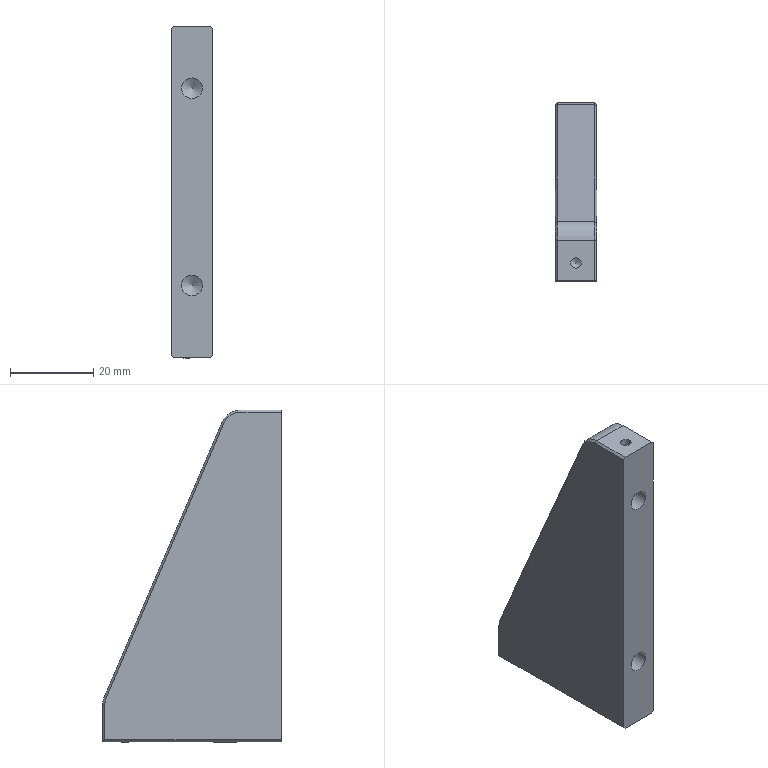Part | STEP file | ROTATION MC_NEW VER-0610_566 | 1 solid | 33 faces | box 10 x 43 x 80 mm | volume 22787 mm3 | plane 15 | cone 10 | cylinder 8 | commonest cylinder face diameters 5 x4 2.5 x2 10 x2
STEP:
#1=CARTESIAN_POINT('',(-187.469,717.468,-130.341));
#2=VERTEX_POINT('',#1);
#3=CARTESIAN_POINT('',(-187.469,717.468,-132.841));
#4=VERTEX_POINT('',#3);
#5=CARTESIAN_POINT('',(-187.469,717.468,-131.591));
#6=DIRECTION('',(0.,-1.,0.));
#7=DIRECTION('',(0.,0.,1.));
#8=AXIS2_PLACEMENT_3D('',#5,#6,#7);
#9=CIRCLE('',#8,1.25);
#10=EDGE_CURVE('',#2,#4,#9,.T.);
#11=ORIENTED_EDGE('',*,*,#10,.F.);
#12=CARTESIAN_POINT('',(-187.469,717.468,-131.591));
#13=DIRECTION('',(0.,-1.,0.));
#14=DIRECTION('',(0.,0.,1.));
#15=AXIS2_PLACEMENT_3D('',#12,#13,#14);
#16=CIRCLE('',#15,1.25);
#17=EDGE_CURVE('',#4,#2,#16,.T.);
#18=ORIENTED_EDGE('',*,*,#17,.F.);
#19=CARTESIAN_POINT('',(-187.469,712.468,-132.841));
#20=VERTEX_POINT('',#19);
#21=CARTESIAN_POINT('',(-187.469,717.468,-132.841));
#22=DIRECTION('',(0.,-1.,0.));
#23=VECTOR('',#22,1.25);
#24=LINE('',#21,#23);
#25=EDGE_CURVE('',#4,#20,#24,.T.);
#26=ORIENTED_EDGE('',*,*,#25,.T.);
#27=CARTESIAN_POINT('',(-187.469,712.468,-130.341));
#28=VERTEX_POINT('',#27);
#29=CARTESIAN_POINT('',(-187.469,712.468,-131.591));
#30=DIRECTION('',(0.,1.,0.));
#31=DIRECTION('',(0.,0.,1.));
#32=AXIS2_PLACEMENT_3D('',#29,#30,#31);
#33=CIRCLE('',#32,1.25);
#34=EDGE_CURVE('',#28,#20,#33,.T.);
#35=ORIENTED_EDGE('',*,*,#34,.F.);
#36=CARTESIAN_POINT('',(-187.469,712.468,-131.591));
#37=DIRECTION('',(0.,1.,0.));
#38=DIRECTION('',(0.,0.,1.));
#39=AXIS2_PLACEMENT_3D('',#36,#37,#38);
#40=CIRCLE('',#39,1.25);
#41=EDGE_CURVE('',#20,#28,#40,.T.);
#42=ORIENTED_EDGE('',*,*,#41,.F.);
#43=ORIENTED_EDGE('',*,*,#25,.F.);
#44=EDGE_LOOP('',(#11,#18,#26,#35,#42,#43));
#45=FACE_OUTER_BOUND('',#44,.T.);
#46=CARTESIAN_POINT('',(-187.469,717.468,-131.591));
#47=DIRECTION('',(0.,-1.,0.));
#48=DIRECTION('',(0.,0.,1.));
#49=AXIS2_PLACEMENT_3D('',#46,#47,#48);
#50=CYLINDRICAL_SURFACE('',#49,1.25);
#51=ADVANCED_FACE('',(#45),#50,.F.);
#52=CARTESIAN_POINT('',(-187.469,711.717,-131.591));
#53=VERTEX_POINT('',#52);
#54=CARTESIAN_POINT('',(-187.469,712.468,-130.341));
#55=DIRECTION('',(0.,0.515,0.8572));
#56=VECTOR('',#55,1.25);
#57=LINE('',#54,#56);
#58=EDGE_CURVE('',#53,#28,#57,.T.);
#59=ORIENTED_EDGE('',*,*,#58,.T.);
#60=ORIENTED_EDGE('',*,*,#34,.T.);
#61=ORIENTED_EDGE('',*,*,#41,.T.);
#62=ORIENTED_EDGE('',*,*,#58,.F.);
#63=EDGE_LOOP('',(#59,#60,#61,#62));
#64=FACE_OUTER_BOUND('',#63,.T.);
#65=CARTESIAN_POINT('',(-187.469,712.468,-131.591));
#66=DIRECTION('',(0.,1.,0.));
#67=DIRECTION('',(0.,0.,-1.));
#68=AXIS2_PLACEMENT_3D('',#65,#66,#67);
#69=CONICAL_SURFACE('',#68,1.25,1.03);
#70=ADVANCED_FACE('',(#64),#69,.F.);
#71=CARTESIAN_POINT('',(-187.469,685.468,-136.091));
#72=VERTEX_POINT('',#71);
#73=CARTESIAN_POINT('',(-187.469,680.468,-136.091));
#74=VERTEX_POINT('',#73);
#75=CARTESIAN_POINT('',(-187.469,682.968,-136.091));
#76=DIRECTION('',(0.,0.,1.));
#77=DIRECTION('',(0.,1.,0.));
#78=AXIS2_PLACEMENT_3D('',#75,#76,#77);
#79=CIRCLE('',#78,2.5);
#80=EDGE_CURVE('',#72,#74,#79,.T.);
#81=ORIENTED_EDGE('',*,*,#80,.F.);
#82=CARTESIAN_POINT('',(-187.469,682.968,-136.091));
#83=DIRECTION('',(0.,0.,1.));
#84=DIRECTION('',(0.,1.,0.));
#85=AXIS2_PLACEMENT_3D('',#82,#83,#84);
#86=CIRCLE('',#85,2.5);
#87=EDGE_CURVE('',#74,#72,#86,.T.);
#88=ORIENTED_EDGE('',*,*,#87,.F.);
#89=CARTESIAN_POINT('',(-187.469,680.468,-124.091));
#90=VERTEX_POINT('',#89);
#91=CARTESIAN_POINT('',(-187.469,680.468,-136.091));
#92=DIRECTION('',(0.,0.,1.));
#93=VECTOR('',#92,2.5);
#94=LINE('',#91,#93);
#95=EDGE_CURVE('',#74,#90,#94,.T.);
#96=ORIENTED_EDGE('',*,*,#95,.T.);
#97=CARTESIAN_POINT('',(-187.469,685.468,-124.091));
#98=VERTEX_POINT('',#97);
#99=CARTESIAN_POINT('',(-187.469,682.968,-124.091));
#100=DIRECTION('',(0.,0.,-1.));
#101=DIRECTION('',(0.,1.,0.));
#102=AXIS2_PLACEMENT_3D('',#99,#100,#101);
#103=CIRCLE('',#102,2.5);
#104=EDGE_CURVE('',#98,#90,#103,.T.);
#105=ORIENTED_EDGE('',*,*,#104,.F.);
#106=CARTESIAN_POINT('',(-187.469,682.968,-124.091));
#107=DIRECTION('',(0.,0.,-1.));
#108=DIRECTION('',(0.,1.,0.));
#109=AXIS2_PLACEMENT_3D('',#106,#107,#108);
#110=CIRCLE('',#109,2.5);
#111=EDGE_CURVE('',#90,#98,#110,.T.);
#112=ORIENTED_EDGE('',*,*,#111,.F.);
#113=ORIENTED_EDGE('',*,*,#95,.F.);
#114=EDGE_LOOP('',(#81,#88,#96,#105,#112,#113));
#115=FACE_OUTER_BOUND('',#114,.T.);
#116=CARTESIAN_POINT('',(-187.469,682.968,-136.091));
#117=DIRECTION('',(0.,0.,1.));
#118=DIRECTION('',(0.,1.,0.));
#119=AXIS2_PLACEMENT_3D('',#116,#117,#118);
#120=CYLINDRICAL_SURFACE('',#119,2.5);
#121=ADVANCED_FACE('',(#115),#120,.F.);
#122=CARTESIAN_POINT('',(-187.469,682.968,-122.589));
#123=VERTEX_POINT('',#122);
#124=CARTESIAN_POINT('',(-187.469,685.468,-124.091));
#125=DIRECTION('',(0.,0.8572,-0.515));
#126=VECTOR('',#125,2.5);
#127=LINE('',#124,#126);
#128=EDGE_CURVE('',#123,#98,#127,.T.);
#129=ORIENTED_EDGE('',*,*,#128,.T.);
#130=ORIENTED_EDGE('',*,*,#104,.T.);
#131=ORIENTED_EDGE('',*,*,#111,.T.);
#132=ORIENTED_EDGE('',*,*,#128,.F.);
#133=EDGE_LOOP('',(#129,#130,#131,#132));
#134=FACE_OUTER_BOUND('',#133,.T.);
#135=CARTESIAN_POINT('',(-187.469,682.968,-124.091));
#136=DIRECTION('',(0.,0.,-1.));
#137=DIRECTION('',(0.,-1.,0.));
#138=AXIS2_PLACEMENT_3D('',#135,#136,#137);
#139=CONICAL_SURFACE('',#138,2.5,1.03);
#140=ADVANCED_FACE('',(#134),#139,.F.);
#141=CARTESIAN_POINT('',(-187.469,711.468,-136.091));
#142=VERTEX_POINT('',#141);
#143=CARTESIAN_POINT('',(-187.469,706.468,-136.091));
#144=VERTEX_POINT('',#143);
#145=CARTESIAN_POINT('',(-187.469,708.968,-136.091));
#146=DIRECTION('',(0.,0.,1.));
#147=DIRECTION('',(0.,1.,0.));
#148=AXIS2_PLACEMENT_3D('',#145,#146,#147);
#149=CIRCLE('',#148,2.5);
#150=EDGE_CURVE('',#142,#144,#149,.T.);
#151=ORIENTED_EDGE('',*,*,#150,.F.);
#152=CARTESIAN_POINT('',(-187.469,708.968,-136.091));
#153=DIRECTION('',(0.,0.,1.));
#154=DIRECTION('',(0.,1.,0.));
#155=AXIS2_PLACEMENT_3D('',#152,#153,#154);
#156=CIRCLE('',#155,2.5);
#157=EDGE_CURVE('',#144,#142,#156,.T.);
#158=ORIENTED_EDGE('',*,*,#157,.F.);
#159=CARTESIAN_POINT('',(-187.469,706.468,-124.091));
#160=VERTEX_POINT('',#159);
#161=CARTESIAN_POINT('',(-187.469,706.468,-136.091));
#162=DIRECTION('',(0.,0.,1.));
#163=VECTOR('',#162,2.5);
#164=LINE('',#161,#163);
#165=EDGE_CURVE('',#144,#160,#164,.T.);
#166=ORIENTED_EDGE('',*,*,#165,.T.);
#167=CARTESIAN_POINT('',(-187.469,711.468,-124.091));
#168=VERTEX_POINT('',#167);
#169=CARTESIAN_POINT('',(-187.469,708.968,-124.091));
#170=DIRECTION('',(0.,0.,-1.));
#171=DIRECTION('',(0.,1.,0.));
#172=AXIS2_PLACEMENT_3D('',#169,#170,#171);
#173=CIRCLE('',#172,2.5);
#174=EDGE_CURVE('',#168,#160,#173,.T.);
#175=ORIENTED_EDGE('',*,*,#174,.F.);
#176=CARTESIAN_POINT('',(-187.469,708.968,-124.091));
#177=DIRECTION('',(0.,0.,-1.));
#178=DIRECTION('',(0.,1.,0.));
#179=AXIS2_PLACEMENT_3D('',#176,#177,#178);
#180=CIRCLE('',#179,2.5);
#181=EDGE_CURVE('',#160,#168,#180,.T.);
#182=ORIENTED_EDGE('',*,*,#181,.F.);
#183=ORIENTED_EDGE('',*,*,#165,.F.);
#184=EDGE_LOOP('',(#151,#158,#166,#175,#182,#183));
#185=FACE_OUTER_BOUND('',#184,.T.);
#186=CARTESIAN_POINT('',(-187.469,708.968,-136.091));
#187=DIRECTION('',(0.,0.,1.));
#188=DIRECTION('',(0.,1.,0.));
#189=AXIS2_PLACEMENT_3D('',#186,#187,#188);
#190=CYLINDRICAL_SURFACE('',#189,2.5);
#191=ADVANCED_FACE('',(#185),#190,.F.);
#192=CARTESIAN_POINT('',(-187.469,708.968,-122.589));
#193=VERTEX_POINT('',#192);
#194=CARTESIAN_POINT('',(-187.469,711.468,-124.091));
#195=DIRECTION('',(0.,0.8572,-0.515));
#196=VECTOR('',#195,2.5);
#197=LINE('',#194,#196);
#198=EDGE_CURVE('',#193,#168,#197,.T.);
#199=ORIENTED_EDGE('',*,*,#198,.T.);
#200=ORIENTED_EDGE('',*,*,#174,.T.);
#201=ORIENTED_EDGE('',*,*,#181,.T.);
#202=ORIENTED_EDGE('',*,*,#198,.F.);
#203=EDGE_LOOP('',(#199,#200,#201,#202));
#204=FACE_OUTER_BOUND('',#203,.T.);
#205=CARTESIAN_POINT('',(-187.469,708.968,-124.091));
#206=DIRECTION('',(0.,0.,-1.));
#207=DIRECTION('',(0.,-1.,0.));
#208=AXIS2_PLACEMENT_3D('',#205,#206,#207);
#209=CONICAL_SURFACE('',#208,2.5,1.03);
#210=ADVANCED_FACE('',(#204),#209,.F.);
#211=CARTESIAN_POINT('',(-187.469,674.468,-121.091));
#212=VERTEX_POINT('',#211);
#213=CARTESIAN_POINT('',(-187.469,674.468,-116.091));
#214=VERTEX_POINT('',#213);
#215=CARTESIAN_POINT('',(-187.469,674.468,-118.591));
#216=DIRECTION('',(0.,1.,0.));
#217=DIRECTION('',(0.,0.,-1.));
#218=AXIS2_PLACEMENT_3D('',#215,#216,#217);
#219=CIRCLE('',#218,2.5);
#220=EDGE_CURVE('',#212,#214,#219,.T.);
#221=ORIENTED_EDGE('',*,*,#220,.F.);
#222=CARTESIAN_POINT('',(-187.469,674.468,-118.591));
#223=DIRECTION('',(0.,1.,0.));
#224=DIRECTION('',(0.,0.,-1.));
#225=AXIS2_PLACEMENT_3D('',#222,#223,#224);
#226=CIRCLE('',#225,2.5);
#227=EDGE_CURVE('',#214,#212,#226,.T.);
#228=ORIENTED_EDGE('',*,*,#227,.F.);
#229=CARTESIAN_POINT('',(-187.469,686.468,-116.091));
#230=VERTEX_POINT('',#229);
#231=CARTESIAN_POINT('',(-187.469,674.468,-116.091));
#232=DIRECTION('',(0.,1.,0.));
#233=VECTOR('',#232,2.5);
#234=LINE('',#231,#233);
#235=EDGE_CURVE('',#214,#230,#234,.T.);
#236=ORIENTED_EDGE('',*,*,#235,.T.);
#237=CARTESIAN_POINT('',(-187.469,686.468,-121.091));
#238=VERTEX_POINT('',#237);
#239=CARTESIAN_POINT('',(-187.469,686.468,-118.591));
#240=DIRECTION('',(0.,-1.,0.));
#241=DIRECTION('',(0.,0.,-1.));
#242=AXIS2_PLACEMENT_3D('',#239,#240,#241);
#243=CIRCLE('',#242,2.5);
#244=EDGE_CURVE('',#238,#230,#243,.T.);
#245=ORIENTED_EDGE('',*,*,#244,.F.);
#246=CARTESIAN_POINT('',(-187.469,686.468,-118.591));
#247=DIRECTION('',(0.,-1.,0.));
#248=DIRECTION('',(0.,0.,-1.));
#249=AXIS2_PLACEMENT_3D('',#246,#247,#248);
#250=CIRCLE('',#249,2.5);
#251=EDGE_CURVE('',#230,#238,#250,.T.);
#252=ORIENTED_EDGE('',*,*,#251,.F.);
#253=ORIENTED_EDGE('',*,*,#235,.F.);
#254=EDGE_LOOP('',(#221,#228,#236,#245,#252,#253));
#255=FACE_OUTER_BOUND('',#254,.T.);
#256=CARTESIAN_POINT('',(-187.469,674.468,-118.591));
#257=DIRECTION('',(0.,1.,0.));
#258=DIRECTION('',(0.,0.,-1.));
#259=AXIS2_PLACEMENT_3D('',#256,#257,#258);
#260=CYLINDRICAL_SURFACE('',#259,2.5);
#261=ADVANCED_FACE('',(#255),#260,.F.);
#262=CARTESIAN_POINT('',(-187.469,687.971,-118.591));
#263=VERTEX_POINT('',#262);
#264=CARTESIAN_POINT('',(-187.469,686.468,-121.091));
#265=DIRECTION('',(0.,-0.515,-0.8572));
#266=VECTOR('',#265,2.5);
#267=LINE('',#264,#266);
#268=EDGE_CURVE('',#263,#238,#267,.T.);
#269=ORIENTED_EDGE('',*,*,#268,.T.);
#270=ORIENTED_EDGE('',*,*,#244,.T.);
#271=ORIENTED_EDGE('',*,*,#251,.T.);
#272=ORIENTED_EDGE('',*,*,#268,.F.);
#273=EDGE_LOOP('',(#269,#270,#271,#272));
#274=FACE_OUTER_BOUND('',#273,.T.);
#275=CARTESIAN_POINT('',(-187.469,686.468,-118.591));
#276=DIRECTION('',(0.,-1.,0.));
#277=DIRECTION('',(0.,0.,1.));
#278=AXIS2_PLACEMENT_3D('',#275,#276,#277);
#279=CONICAL_SURFACE('',#278,2.5,1.03);
#280=ADVANCED_FACE('',(#274),#279,.F.);
#281=CARTESIAN_POINT('',(-187.469,674.468,-73.591));
#282=VERTEX_POINT('',#281);
#283=CARTESIAN_POINT('',(-187.469,674.468,-68.591));
#284=VERTEX_POINT('',#283);
#285=CARTESIAN_POINT('',(-187.469,674.468,-71.091));
#286=DIRECTION('',(0.,1.,0.));
#287=DIRECTION('',(0.,0.,-1.));
#288=AXIS2_PLACEMENT_3D('',#285,#286,#287);
#289=CIRCLE('',#288,2.5);
#290=EDGE_CURVE('',#282,#284,#289,.T.);
#291=ORIENTED_EDGE('',*,*,#290,.F.);
#292=CARTESIAN_POINT('',(-187.469,674.468,-71.091));
#293=DIRECTION('',(0.,1.,0.));
#294=DIRECTION('',(0.,0.,-1.));
#295=AXIS2_PLACEMENT_3D('',#292,#293,#294);
#296=CIRCLE('',#295,2.5);
#297=EDGE_CURVE('',#284,#282,#296,.T.);
#298=ORIENTED_EDGE('',*,*,#297,.F.);
#299=CARTESIAN_POINT('',(-187.469,686.468,-68.591));
#300=VERTEX_POINT('',#299);
#301=CARTESIAN_POINT('',(-187.469,674.468,-68.591));
#302=DIRECTION('',(0.,1.,0.));
#303=VECTOR('',#302,2.5);
#304=LINE('',#301,#303);
#305=EDGE_CURVE('',#284,#300,#304,.T.);
#306=ORIENTED_EDGE('',*,*,#305,.T.);
#307=CARTESIAN_POINT('',(-187.469,686.468,-73.591));
#308=VERTEX_POINT('',#307);
#309=CARTESIAN_POINT('',(-187.469,686.468,-71.091));
#310=DIRECTION('',(0.,-1.,0.));
#311=DIRECTION('',(0.,0.,-1.));
#312=AXIS2_PLACEMENT_3D('',#309,#310,#311);
#313=CIRCLE('',#312,2.5);
#314=EDGE_CURVE('',#308,#300,#313,.T.);
#315=ORIENTED_EDGE('',*,*,#314,.F.);
#316=CARTESIAN_POINT('',(-187.469,686.468,-71.091));
#317=DIRECTION('',(0.,-1.,0.));
#318=DIRECTION('',(0.,0.,-1.));
#319=AXIS2_PLACEMENT_3D('',#316,#317,#318);
#320=CIRCLE('',#319,2.5);
#321=EDGE_CURVE('',#300,#308,#320,.T.);
#322=ORIENTED_EDGE('',*,*,#321,.F.);
#323=ORIENTED_EDGE('',*,*,#305,.F.);
#324=EDGE_LOOP('',(#291,#298,#306,#315,#322,#323));
#325=FACE_OUTER_BOUND('',#324,.T.);
#326=CARTESIAN_POINT('',(-187.469,674.468,-71.091));
#327=DIRECTION('',(0.,1.,0.));
#328=DIRECTION('',(0.,0.,-1.));
#329=AXIS2_PLACEMENT_3D('',#326,#327,#328);
#330=CYLINDRICAL_SURFACE('',#329,2.5);
#331=ADVANCED_FACE('',(#325),#330,.F.);
#332=CARTESIAN_POINT('',(-187.469,687.971,-71.091));
#333=VERTEX_POINT('',#332);
#334=CARTESIAN_POINT('',(-187.469,686.468,-73.591));
#335=DIRECTION('',(0.,-0.515,-0.8572));
#336=VECTOR('',#335,2.5);
#337=LINE('',#334,#336);
#338=EDGE_CURVE('',#333,#308,#337,.T.);
#339=ORIENTED_EDGE('',*,*,#338,.T.);
#340=ORIENTED_EDGE('',*,*,#314,.T.);
#341=ORIENTED_EDGE('',*,*,#321,.T.);
#342=ORIENTED_EDGE('',*,*,#338,.F.);
#343=EDGE_LOOP('',(#339,#340,#341,#342));
#344=FACE_OUTER_BOUND('',#343,.T.);
#345=CARTESIAN_POINT('',(-187.469,686.468,-71.091));
#346=DIRECTION('',(0.,-1.,0.));
#347=DIRECTION('',(0.,0.,1.));
#348=AXIS2_PLACEMENT_3D('',#345,#346,#347);
#349=CONICAL_SURFACE('',#348,2.5,1.03);
#350=ADVANCED_FACE('',(#344),#349,.F.);
#351=CARTESIAN_POINT('',(-186.219,678.718,-56.091));
#352=VERTEX_POINT('',#351);
#353=CARTESIAN_POINT('',(-188.719,678.718,-56.091));
#354=VERTEX_POINT('',#353);
#355=CARTESIAN_POINT('',(-187.469,678.718,-56.091));
#356=DIRECTION('',(0.,0.,-1.));
#357=DIRECTION('',(1.,0.,0.));
#358=AXIS2_PLACEMENT_3D('',#355,#356,#357);
#359=CIRCLE('',#358,1.25);
#360=EDGE_CURVE('',#352,#354,#359,.T.);
#361=ORIENTED_EDGE('',*,*,#360,.F.);
#362=CARTESIAN_POINT('',(-187.469,678.718,-56.091));
#363=DIRECTION('',(0.,0.,-1.));
#364=DIRECTION('',(1.,0.,0.));
#365=AXIS2_PLACEMENT_3D('',#362,#363,#364);
#366=CIRCLE('',#365,1.25);
#367=EDGE_CURVE('',#354,#352,#366,.T.);
#368=ORIENTED_EDGE('',*,*,#367,.F.);
#369=CARTESIAN_POINT('',(-188.719,678.718,-66.091));
#370=VERTEX_POINT('',#369);
#371=CARTESIAN_POINT('',(-188.719,678.718,-56.091));
#372=DIRECTION('',(0.,0.,-1.));
#373=VECTOR('',#372,1.25);
#374=LINE('',#371,#373);
#375=EDGE_CURVE('',#354,#370,#374,.T.);
#376=ORIENTED_EDGE('',*,*,#375,.T.);
#377=CARTESIAN_POINT('',(-186.219,678.718,-66.091));
#378=VERTEX_POINT('',#377);
#379=CARTESIAN_POINT('',(-187.469,678.718,-66.091));
#380=DIRECTION('',(0.,0.,1.));
#381=DIRECTION('',(1.,0.,0.));
#382=AXIS2_PLACEMENT_3D('',#379,#380,#381);
#383=CIRCLE('',#382,1.25);
#384=EDGE_CURVE('',#378,#370,#383,.T.);
#385=ORIENTED_EDGE('',*,*,#384,.F.);
#386=CARTESIAN_POINT('',(-187.469,678.718,-66.091));
#387=DIRECTION('',(0.,0.,1.));
#388=DIRECTION('',(1.,0.,0.));
#389=AXIS2_PLACEMENT_3D('',#386,#387,#388);
#390=CIRCLE('',#389,1.25);
#391=EDGE_CURVE('',#370,#378,#390,.T.);
#392=ORIENTED_EDGE('',*,*,#391,.F.);
#393=ORIENTED_EDGE('',*,*,#375,.F.);
#394=EDGE_LOOP('',(#361,#368,#376,#385,#392,#393));
#395=FACE_OUTER_BOUND('',#394,.T.);
#396=CARTESIAN_POINT('',(-187.469,678.718,-56.091));
#397=DIRECTION('',(0.,0.,-1.));
#398=DIRECTION('',(1.,0.,0.));
#399=AXIS2_PLACEMENT_3D('',#396,#397,#398);
#400=CYLINDRICAL_SURFACE('',#399,1.25);
#401=ADVANCED_FACE('',(#395),#400,.F.);
#402=CARTESIAN_POINT('',(-187.469,678.718,-66.842));
#403=VERTEX_POINT('',#402);
#404=CARTESIAN_POINT('',(-186.219,678.718,-66.091));
#405=DIRECTION('',(0.8572,0.,0.515));
#406=VECTOR('',#405,1.25);
#407=LINE('',#404,#406);
#408=EDGE_CURVE('',#403,#378,#407,.T.);
#409=ORIENTED_EDGE('',*,*,#408,.T.);
#410=ORIENTED_EDGE('',*,*,#384,.T.);
#411=ORIENTED_EDGE('',*,*,#391,.T.);
#412=ORIENTED_EDGE('',*,*,#408,.F.);
#413=EDGE_LOOP('',(#409,#410,#411,#412));
#414=FACE_OUTER_BOUND('',#413,.T.);
#415=CARTESIAN_POINT('',(-187.469,678.718,-66.091));
#416=DIRECTION('',(0.,0.,1.));
#417=DIRECTION('',(-1.,0.,0.));
#418=AXIS2_PLACEMENT_3D('',#415,#416,#417);
#419=CONICAL_SURFACE('',#418,1.25,1.03);
#420=ADVANCED_FACE('',(#414),#419,.F.);
#421=CARTESIAN_POINT('',(-182.969,674.468,-56.091));
#422=VERTEX_POINT('',#421);
#423=CARTESIAN_POINT('',(-182.969,684.171,-56.091));
#424=VERTEX_POINT('',#423);
#425=CARTESIAN_POINT('',(-182.969,674.468,-56.091));
#426=DIRECTION('',(0.,1.,0.));
#427=VECTOR('',#426,9.703);
#428=LINE('',#425,#427);
#429=EDGE_CURVE('',#422,#424,#428,.T.);
#430=ORIENTED_EDGE('',*,*,#429,.T.);
#431=CARTESIAN_POINT('',(-191.969,684.171,-56.091));
#432=VERTEX_POINT('',#431);
#433=CARTESIAN_POINT('',(-191.969,684.171,-56.091));
#434=DIRECTION('',(1.,0.,0.));
#435=VECTOR('',#434,9.);
#436=LINE('',#433,#435);
#437=EDGE_CURVE('',#432,#424,#436,.T.);
#438=ORIENTED_EDGE('',*,*,#437,.F.);
#439=CARTESIAN_POINT('',(-191.969,674.468,-56.091));
#440=VERTEX_POINT('',#439);
#441=CARTESIAN_POINT('',(-191.969,684.171,-56.091));
#442=DIRECTION('',(0.,-1.,0.));
#443=VECTOR('',#442,9.703);
#444=LINE('',#441,#443);
#445=EDGE_CURVE('',#432,#440,#444,.T.);
#446=ORIENTED_EDGE('',*,*,#445,.T.);
#447=CARTESIAN_POINT('',(-191.969,674.468,-56.091));
#448=DIRECTION('',(1.,0.,0.));
#449=VECTOR('',#448,9.);
#450=LINE('',#447,#449);
#451=EDGE_CURVE('',#440,#422,#450,.T.);
#452=ORIENTED_EDGE('',*,*,#451,.T.);
#453=EDGE_LOOP('',(#430,#438,#446,#452));
#454=FACE_OUTER_BOUND('',#453,.T.);
#455=ORIENTED_EDGE('',*,*,#360,.T.);
#456=ORIENTED_EDGE('',*,*,#367,.T.);
#457=EDGE_LOOP('',(#455,#456));
#458=FACE_BOUND('',#457,.T.);
#459=CARTESIAN_POINT('',(-179.469,848.159,-56.091));
#460=DIRECTION('',(0.,0.,1.));
#461=DIRECTION('',(1.,0.,0.));
#462=AXIS2_PLACEMENT_3D('',#459,#460,#461);
#463=PLANE('',#462);
#464=ADVANCED_FACE('',(#454,#458),#463,.T.);
#465=CARTESIAN_POINT('',(-182.469,674.468,-56.591));
#466=VERTEX_POINT('',#465);
#467=CARTESIAN_POINT('',(-182.469,674.468,-56.591));
#468=DIRECTION('',(-0.7071,0.,0.7071));
#469=VECTOR('',#468,0.7071);
#470=LINE('',#467,#469);
#471=EDGE_CURVE('',#466,#422,#470,.T.);
#472=ORIENTED_EDGE('',*,*,#471,.F.);
#473=CARTESIAN_POINT('',(-182.469,684.171,-56.591));
#474=VERTEX_POINT('',#473);
#475=CARTESIAN_POINT('',(-182.469,684.171,-56.591));
#476=DIRECTION('',(0.,-1.,0.));
#477=VECTOR('',#476,9.703);
#478=LINE('',#475,#477);
#479=EDGE_CURVE('',#474,#466,#478,.T.);
#480=ORIENTED_EDGE('',*,*,#479,.F.);
#481=CARTESIAN_POINT('',(-182.969,684.171,-56.091));
#482=DIRECTION('',(0.7071,0.,-0.7071));
#483=VECTOR('',#482,0.7071);
#484=LINE('',#481,#483);
#485=EDGE_CURVE('',#424,#474,#484,.T.);
#486=ORIENTED_EDGE('',*,*,#485,.F.);
#487=ORIENTED_EDGE('',*,*,#429,.F.);
#488=EDGE_LOOP('',(#472,#480,#486,#487));
#489=FACE_OUTER_BOUND('',#488,.T.);
#490=CARTESIAN_POINT('',(-182.719,755.409,-56.341));
#491=DIRECTION('',(0.7071,0.,0.7071));
#492=DIRECTION('',(0.7071,0.,-0.7071));
#493=AXIS2_PLACEMENT_3D('',#490,#491,#492);
#494=PLANE('',#493);
#495=ADVANCED_FACE('',(#489),#494,.T.);
#496=ORIENTED_EDGE('',*,*,#471,.T.);
#497=ORIENTED_EDGE('',*,*,#451,.F.);
#498=CARTESIAN_POINT('',(-192.469,674.468,-56.591));
#499=VERTEX_POINT('',#498);
#500=CARTESIAN_POINT('',(-191.969,674.468,-56.091));
#501=DIRECTION('',(-0.7071,0.,-0.7071));
#502=VECTOR('',#501,0.7071);
#503=LINE('',#500,#502);
#504=EDGE_CURVE('',#440,#499,#503,.T.);
#505=ORIENTED_EDGE('',*,*,#504,.T.);
#506=CARTESIAN_POINT('',(-192.469,674.468,-135.591));
#507=VERTEX_POINT('',#506);
#508=CARTESIAN_POINT('',(-192.469,674.468,-135.591));
#509=DIRECTION('',(0.,0.,1.));
#510=VECTOR('',#509,79.);
#511=LINE('',#508,#510);
#512=EDGE_CURVE('',#507,#499,#511,.T.);
#513=ORIENTED_EDGE('',*,*,#512,.F.);
#514=CARTESIAN_POINT('',(-191.969,674.468,-136.091));
#515=VERTEX_POINT('',#514);
#516=CARTESIAN_POINT('',(-192.469,674.468,-135.591));
#517=DIRECTION('',(0.7071,0.,-0.7071));
#518=VECTOR('',#517,0.7071);
#519=LINE('',#516,#518);
#520=EDGE_CURVE('',#507,#515,#519,.T.);
#521=ORIENTED_EDGE('',*,*,#520,.T.);
#522=CARTESIAN_POINT('',(-182.969,674.468,-136.091));
#523=VERTEX_POINT('',#522);
#524=CARTESIAN_POINT('',(-182.969,674.468,-136.091));
#525=DIRECTION('',(-1.,0.,0.));
#526=VECTOR('',#525,9.);
#527=LINE('',#524,#526);
#528=EDGE_CURVE('',#523,#515,#527,.T.);
#529=ORIENTED_EDGE('',*,*,#528,.F.);
#530=CARTESIAN_POINT('',(-182.469,674.468,-135.591));
#531=VERTEX_POINT('',#530);
#532=CARTESIAN_POINT('',(-182.969,674.468,-136.091));
#533=DIRECTION('',(0.7071,0.,0.7071));
#534=VECTOR('',#533,0.7071);
#535=LINE('',#532,#534);
#536=EDGE_CURVE('',#523,#531,#535,.T.);
#537=ORIENTED_EDGE('',*,*,#536,.T.);
#538=CARTESIAN_POINT('',(-182.469,674.468,-56.591));
#539=DIRECTION('',(0.,0.,-1.));
#540=VECTOR('',#539,79.);
#541=LINE('',#538,#540);
#542=EDGE_CURVE('',#466,#531,#541,.T.);
#543=ORIENTED_EDGE('',*,*,#542,.F.);
#544=EDGE_LOOP('',(#496,#497,#505,#513,#521,#529,#537,#543));
#545=FACE_OUTER_BOUND('',#544,.T.);
#546=ORIENTED_EDGE('',*,*,#290,.T.);
#547=ORIENTED_EDGE('',*,*,#297,.T.);
#548=EDGE_LOOP('',(#546,#547));
#549=FACE_BOUND('',#548,.T.);
#550=ORIENTED_EDGE('',*,*,#220,.T.);
#551=ORIENTED_EDGE('',*,*,#227,.T.);
#552=EDGE_LOOP('',(#550,#551));
#553=FACE_BOUND('',#552,.T.);
#554=CARTESIAN_POINT('',(-179.469,674.468,-102.091));
#555=DIRECTION('',(0.,-1.,0.));
#556=DIRECTION('',(0.,0.,-1.));
#557=AXIS2_PLACEMENT_3D('',#554,#555,#556);
#558=PLANE('',#557);
#559=ADVANCED_FACE('',(#545,#549,#553),#558,.T.);
#560=ORIENTED_EDGE('',*,*,#479,.T.);
#561=ORIENTED_EDGE('',*,*,#542,.T.);
#562=CARTESIAN_POINT('',(-182.469,716.968,-135.591));
#563=VERTEX_POINT('',#562);
#564=CARTESIAN_POINT('',(-182.469,674.468,-135.591));
#565=DIRECTION('',(0.,1.,0.));
#566=VECTOR('',#565,42.5);
#567=LINE('',#564,#566);
#568=EDGE_CURVE('',#531,#563,#567,.T.);
#569=ORIENTED_EDGE('',*,*,#568,.T.);
#570=CARTESIAN_POINT('',(-182.469,716.968,-127.118));
#571=VERTEX_POINT('',#570);
#572=CARTESIAN_POINT('',(-182.469,716.968,-135.591));
#573=DIRECTION('',(0.,0.,1.));
#574=VECTOR('',#573,8.474);
#575=LINE('',#572,#574);
#576=EDGE_CURVE('',#563,#571,#575,.T.);
#577=ORIENTED_EDGE('',*,*,#576,.T.);
#578=CARTESIAN_POINT('',(-182.469,716.605,-125.345));
#579=VERTEX_POINT('',#578);
#580=CARTESIAN_POINT('',(-182.469,712.468,-127.118));
#581=DIRECTION('',(1.,0.,0.));
#582=DIRECTION('',(0.,1.,0.));
#583=AXIS2_PLACEMENT_3D('',#580,#581,#582);
#584=CIRCLE('',#583,4.5);
#585=EDGE_CURVE('',#571,#579,#584,.T.);
#586=ORIENTED_EDGE('',*,*,#585,.T.);
#587=CARTESIAN_POINT('',(-182.469,688.308,-59.319));
#588=VERTEX_POINT('',#587);
#589=CARTESIAN_POINT('',(-182.469,716.605,-125.345));
#590=DIRECTION('',(0.,-0.3939,0.9191));
#591=VECTOR('',#590,71.834);
#592=LINE('',#589,#591);
#593=EDGE_CURVE('',#579,#588,#592,.T.);
#594=ORIENTED_EDGE('',*,*,#593,.T.);
#595=CARTESIAN_POINT('',(-182.469,684.171,-61.091));
#596=DIRECTION('',(1.,0.,0.));
#597=DIRECTION('',(0.,0.9191,0.3939));
#598=AXIS2_PLACEMENT_3D('',#595,#596,#597);
#599=CIRCLE('',#598,4.5);
#600=EDGE_CURVE('',#588,#474,#599,.T.);
#601=ORIENTED_EDGE('',*,*,#600,.T.);
#602=EDGE_LOOP('',(#560,#561,#569,#577,#586,#594,#601));
#603=FACE_OUTER_BOUND('',#602,.T.);
#604=CARTESIAN_POINT('',(-182.469,662.659,-65.591));
#605=DIRECTION('',(-1.,0.,0.));
#606=DIRECTION('',(0.,0.,1.));
#607=AXIS2_PLACEMENT_3D('',#604,#605,#606);
#608=PLANE('',#607);
#609=ADVANCED_FACE('',(#603),#608,.F.);
#610=ORIENTED_EDGE('',*,*,#600,.F.);
#611=CARTESIAN_POINT('',(-182.969,688.767,-59.122));
#612=VERTEX_POINT('',#611);
#613=CARTESIAN_POINT('',(-182.969,688.767,-59.122));
#614=DIRECTION('',(0.7071,-0.6499,-0.2785));
#615=VECTOR('',#614,0.7071);
#616=LINE('',#613,#615);
#617=EDGE_CURVE('',#612,#588,#616,.T.);
#618=ORIENTED_EDGE('',*,*,#617,.F.);
#619=CARTESIAN_POINT('',(-182.969,684.171,-61.091));
#620=DIRECTION('',(1.,0.,0.));
#621=DIRECTION('',(0.,0.5505,0.8348));
#622=AXIS2_PLACEMENT_3D('',#619,#620,#621);
#623=CIRCLE('',#622,5.);
#624=EDGE_CURVE('',#612,#424,#623,.T.);
#625=ORIENTED_EDGE('',*,*,#624,.T.);
#626=ORIENTED_EDGE('',*,*,#485,.T.);
#627=EDGE_LOOP('',(#610,#618,#625,#626));
#628=FACE_OUTER_BOUND('',#627,.T.);
#629=CARTESIAN_POINT('',(-178.969,684.171,-61.091));
#630=DIRECTION('',(-1.,0.,0.));
#631=DIRECTION('',(0.,0.5505,0.8348));
#632=AXIS2_PLACEMENT_3D('',#629,#630,#631);
#633=CONICAL_SURFACE('',#632,1.,0.7854);
#634=ADVANCED_FACE('',(#628),#633,.T.);
#635=CARTESIAN_POINT('',(-191.969,688.767,-59.122));
#636=VERTEX_POINT('',#635);
#637=CARTESIAN_POINT('',(-191.969,684.171,-61.091));
#638=DIRECTION('',(-1.,0.,0.));
#639=DIRECTION('',(0.,0.5505,0.8348));
#640=AXIS2_PLACEMENT_3D('',#637,#638,#639);
#641=CIRCLE('',#640,5.);
#642=EDGE_CURVE('',#432,#636,#641,.T.);
#643=ORIENTED_EDGE('',*,*,#642,.F.);
#644=ORIENTED_EDGE('',*,*,#437,.T.);
#645=ORIENTED_EDGE('',*,*,#624,.F.);
#646=CARTESIAN_POINT('',(-182.969,688.767,-59.122));
#647=DIRECTION('',(-1.,0.,0.));
#648=VECTOR('',#647,9.);
#649=LINE('',#646,#648);
#650=EDGE_CURVE('',#612,#636,#649,.T.);
#651=ORIENTED_EDGE('',*,*,#650,.T.);
#652=EDGE_LOOP('',(#643,#644,#645,#651));
#653=FACE_OUTER_BOUND('',#652,.T.);
#654=CARTESIAN_POINT('',(-179.469,684.171,-61.091));
#655=DIRECTION('',(1.,0.,0.));
#656=DIRECTION('',(0.,0.5505,0.8348));
#657=AXIS2_PLACEMENT_3D('',#654,#655,#656);
#658=CYLINDRICAL_SURFACE('',#657,5.);
#659=ADVANCED_FACE('',(#653),#658,.T.);
#660=CARTESIAN_POINT('',(-192.469,684.171,-56.591));
#661=VERTEX_POINT('',#660);
#662=CARTESIAN_POINT('',(-192.469,688.308,-59.319));
#663=VERTEX_POINT('',#662);
#664=CARTESIAN_POINT('',(-192.469,684.171,-61.091));
#665=DIRECTION('',(-1.,0.,0.));
#666=DIRECTION('',(0.,0.,1.));
#667=AXIS2_PLACEMENT_3D('',#664,#665,#666);
#668=CIRCLE('',#667,4.5);
#669=EDGE_CURVE('',#661,#663,#668,.T.);
#670=ORIENTED_EDGE('',*,*,#669,.F.);
#671=CARTESIAN_POINT('',(-192.469,684.171,-56.591));
#672=DIRECTION('',(0.7071,0.,0.7071));
#673=VECTOR('',#672,0.7071);
#674=LINE('',#671,#673);
#675=EDGE_CURVE('',#661,#432,#674,.T.);
#676=ORIENTED_EDGE('',*,*,#675,.T.);
#677=ORIENTED_EDGE('',*,*,#642,.T.);
#678=CARTESIAN_POINT('',(-191.969,688.767,-59.122));
#679=DIRECTION('',(-0.7071,-0.6499,-0.2785));
#680=VECTOR('',#679,0.7071);
#681=LINE('',#678,#680);
#682=EDGE_CURVE('',#636,#663,#681,.T.);
#683=ORIENTED_EDGE('',*,*,#682,.T.);
#684=EDGE_LOOP('',(#670,#676,#677,#683));
#685=FACE_OUTER_BOUND('',#684,.T.);
#686=CARTESIAN_POINT('',(-195.969,684.171,-61.091));
#687=DIRECTION('',(1.,0.,0.));
#688=DIRECTION('',(0.,0.5505,0.8348));
#689=AXIS2_PLACEMENT_3D('',#686,#687,#688);
#690=CONICAL_SURFACE('',#689,1.,0.7854);
#691=ADVANCED_FACE('',(#685),#690,.T.);
#692=CARTESIAN_POINT('',(-192.469,674.468,-56.591));
#693=DIRECTION('',(0.,1.,0.));
#694=VECTOR('',#693,9.703);
#695=LINE('',#692,#694);
#696=EDGE_CURVE('',#499,#661,#695,.T.);
#697=ORIENTED_EDGE('',*,*,#696,.T.);
#698=ORIENTED_EDGE('',*,*,#669,.T.);
#699=CARTESIAN_POINT('',(-192.469,716.605,-125.345));
#700=VERTEX_POINT('',#699);
#701=CARTESIAN_POINT('',(-192.469,688.308,-59.319));
#702=DIRECTION('',(0.,0.3939,-0.9191));
#703=VECTOR('',#702,71.834);
#704=LINE('',#701,#703);
#705=EDGE_CURVE('',#663,#700,#704,.T.);
#706=ORIENTED_EDGE('',*,*,#705,.T.);
#707=CARTESIAN_POINT('',(-192.469,716.968,-127.118));
#708=VERTEX_POINT('',#707);
#709=CARTESIAN_POINT('',(-192.469,712.468,-127.118));
#710=DIRECTION('',(-1.,0.,0.));
#711=DIRECTION('',(0.,0.9191,0.3939));
#712=AXIS2_PLACEMENT_3D('',#709,#710,#711);
#713=CIRCLE('',#712,4.5);
#714=EDGE_CURVE('',#700,#708,#713,.T.);
#715=ORIENTED_EDGE('',*,*,#714,.T.);
#716=CARTESIAN_POINT('',(-192.469,716.968,-135.591));
#717=VERTEX_POINT('',#716);
#718=CARTESIAN_POINT('',(-192.469,716.968,-127.118));
#719=DIRECTION('',(0.,0.,-1.));
#720=VECTOR('',#719,8.474);
#721=LINE('',#718,#720);
#722=EDGE_CURVE('',#708,#717,#721,.T.);
#723=ORIENTED_EDGE('',*,*,#722,.T.);
#724=CARTESIAN_POINT('',(-192.469,716.968,-135.591));
#725=DIRECTION('',(0.,-1.,0.));
#726=VECTOR('',#725,42.5);
#727=LINE('',#724,#726);
#728=EDGE_CURVE('',#717,#507,#727,.T.);
#729=ORIENTED_EDGE('',*,*,#728,.T.);
#730=ORIENTED_EDGE('',*,*,#512,.T.);
#731=EDGE_LOOP('',(#697,#698,#706,#715,#723,#729,#730));
#732=FACE_OUTER_BOUND('',#731,.T.);
#733=CARTESIAN_POINT('',(-192.469,662.659,-65.591));
#734=DIRECTION('',(-1.,0.,0.));
#735=DIRECTION('',(0.,0.,1.));
#736=AXIS2_PLACEMENT_3D('',#733,#734,#735);
#737=PLANE('',#736);
#738=ADVANCED_FACE('',(#732),#737,.T.);
#739=ORIENTED_EDGE('',*,*,#504,.F.);
#740=ORIENTED_EDGE('',*,*,#445,.F.);
#741=ORIENTED_EDGE('',*,*,#675,.F.);
#742=ORIENTED_EDGE('',*,*,#696,.F.);
#743=EDGE_LOOP('',(#739,#740,#741,#742));
#744=FACE_OUTER_BOUND('',#743,.T.);
#745=CARTESIAN_POINT('',(-192.219,755.409,-56.341));
#746=DIRECTION('',(-0.7071,0.,0.7071));
#747=DIRECTION('',(0.7071,0.,0.7071));
#748=AXIS2_PLACEMENT_3D('',#745,#746,#747);
#749=PLANE('',#748);
#750=ADVANCED_FACE('',(#744),#749,.T.);
#751=ORIENTED_EDGE('',*,*,#520,.F.);
#752=ORIENTED_EDGE('',*,*,#728,.F.);
#753=CARTESIAN_POINT('',(-191.969,717.468,-136.091));
#754=VERTEX_POINT('',#753);
#755=CARTESIAN_POINT('',(-191.969,717.468,-136.091));
#756=DIRECTION('',(-0.5774,-0.5774,0.5774));
#757=VECTOR('',#756,0.866);
#758=LINE('',#755,#757);
#759=EDGE_CURVE('',#754,#717,#758,.T.);
#760=ORIENTED_EDGE('',*,*,#759,.F.);
#761=CARTESIAN_POINT('',(-191.969,674.468,-136.091));
#762=DIRECTION('',(0.,1.,0.));
#763=VECTOR('',#762,43.);
#764=LINE('',#761,#763);
#765=EDGE_CURVE('',#515,#754,#764,.T.);
#766=ORIENTED_EDGE('',*,*,#765,.F.);
#767=EDGE_LOOP('',(#751,#752,#760,#766));
#768=FACE_OUTER_BOUND('',#767,.T.);
#769=CARTESIAN_POINT('',(-192.219,755.409,-135.841));
#770=DIRECTION('',(-0.7071,0.,-0.7071));
#771=DIRECTION('',(-0.7071,0.,0.7071));
#772=AXIS2_PLACEMENT_3D('',#769,#770,#771);
#773=PLANE('',#772);
#774=ADVANCED_FACE('',(#768),#773,.T.);
#775=CARTESIAN_POINT('',(-182.969,717.468,-136.091));
#776=VERTEX_POINT('',#775);
#777=CARTESIAN_POINT('',(-182.969,717.468,-136.091));
#778=DIRECTION('',(0.,-1.,0.));
#779=VECTOR('',#778,43.);
#780=LINE('',#777,#779);
#781=EDGE_CURVE('',#776,#523,#780,.T.);
#782=ORIENTED_EDGE('',*,*,#781,.T.);
#783=ORIENTED_EDGE('',*,*,#528,.T.);
#784=ORIENTED_EDGE('',*,*,#765,.T.);
#785=CARTESIAN_POINT('',(-191.969,717.468,-136.091));
#786=DIRECTION('',(1.,0.,0.));
#787=VECTOR('',#786,9.);
#788=LINE('',#785,#787);
#789=EDGE_CURVE('',#754,#776,#788,.T.);
#790=ORIENTED_EDGE('',*,*,#789,.T.);
#791=EDGE_LOOP('',(#782,#783,#784,#790));
#792=FACE_OUTER_BOUND('',#791,.T.);
#793=ORIENTED_EDGE('',*,*,#150,.T.);
#794=ORIENTED_EDGE('',*,*,#157,.T.);
#795=EDGE_LOOP('',(#793,#794));
#796=FACE_BOUND('',#795,.T.);
#797=ORIENTED_EDGE('',*,*,#80,.T.);
#798=ORIENTED_EDGE('',*,*,#87,.T.);
#799=EDGE_LOOP('',(#797,#798));
#800=FACE_BOUND('',#799,.T.);
#801=CARTESIAN_POINT('',(-179.469,848.159,-136.091));
#802=DIRECTION('',(0.,0.,-1.));
#803=DIRECTION('',(-1.,0.,0.));
#804=AXIS2_PLACEMENT_3D('',#801,#802,#803);
#805=PLANE('',#804);
#806=ADVANCED_FACE('',(#792,#796,#800),#805,.T.);
#807=ORIENTED_EDGE('',*,*,#536,.F.);
#808=ORIENTED_EDGE('',*,*,#781,.F.);
#809=CARTESIAN_POINT('',(-182.969,717.468,-136.091));
#810=DIRECTION('',(0.5774,-0.5774,0.5774));
#811=VECTOR('',#810,0.866);
#812=LINE('',#809,#811);
#813=EDGE_CURVE('',#776,#563,#812,.T.);
#814=ORIENTED_EDGE('',*,*,#813,.T.);
#815=ORIENTED_EDGE('',*,*,#568,.F.);
#816=EDGE_LOOP('',(#807,#808,#814,#815));
#817=FACE_OUTER_BOUND('',#816,.T.);
#818=CARTESIAN_POINT('',(-182.719,755.409,-135.841));
#819=DIRECTION('',(0.7071,0.,-0.7071));
#820=DIRECTION('',(-0.7071,0.,-0.7071));
#821=AXIS2_PLACEMENT_3D('',#818,#819,#820);
#822=PLANE('',#821);
#823=ADVANCED_FACE('',(#817),#822,.T.);
#824=ORIENTED_EDGE('',*,*,#576,.F.);
#825=ORIENTED_EDGE('',*,*,#813,.F.);
#826=CARTESIAN_POINT('',(-182.969,717.468,-127.118));
#827=VERTEX_POINT('',#826);
#828=CARTESIAN_POINT('',(-182.969,717.468,-127.118));
#829=DIRECTION('',(0.,0.,-1.));
#830=VECTOR('',#829,8.974);
#831=LINE('',#828,#830);
#832=EDGE_CURVE('',#827,#776,#831,.T.);
#833=ORIENTED_EDGE('',*,*,#832,.F.);
#834=CARTESIAN_POINT('',(-182.469,716.968,-127.118));
#835=DIRECTION('',(-0.7071,0.7071,0.));
#836=VECTOR('',#835,0.7071);
#837=LINE('',#834,#836);
#838=EDGE_CURVE('',#571,#827,#837,.T.);
#839=ORIENTED_EDGE('',*,*,#838,.F.);
#840=EDGE_LOOP('',(#824,#825,#833,#839));
#841=FACE_OUTER_BOUND('',#840,.T.);
#842=CARTESIAN_POINT('',(-182.719,717.218,-83.841));
#843=DIRECTION('',(0.7071,0.7071,0.));
#844=DIRECTION('',(0.,0.,-1.));
#845=AXIS2_PLACEMENT_3D('',#842,#843,#844);
#846=PLANE('',#845);
#847=ADVANCED_FACE('',(#841),#846,.T.);
#848=ORIENTED_EDGE('',*,*,#585,.F.);
#849=ORIENTED_EDGE('',*,*,#838,.T.);
#850=CARTESIAN_POINT('',(-182.969,717.064,-125.148));
#851=VERTEX_POINT('',#850);
#852=CARTESIAN_POINT('',(-182.969,712.468,-127.118));
#853=DIRECTION('',(1.,0.,0.));
#854=DIRECTION('',(0.,1.,0.));
#855=AXIS2_PLACEMENT_3D('',#852,#853,#854);
#856=CIRCLE('',#855,5.);
#857=EDGE_CURVE('',#827,#851,#856,.T.);
#858=ORIENTED_EDGE('',*,*,#857,.T.);
#859=CARTESIAN_POINT('',(-182.469,716.605,-125.345));
#860=DIRECTION('',(-0.7071,0.6499,0.2785));
#861=VECTOR('',#860,0.7071);
#862=LINE('',#859,#861);
#863=EDGE_CURVE('',#579,#851,#862,.T.);
#864=ORIENTED_EDGE('',*,*,#863,.F.);
#865=EDGE_LOOP('',(#848,#849,#858,#864));
#866=FACE_OUTER_BOUND('',#865,.T.);
#867=CARTESIAN_POINT('',(-178.969,712.468,-127.118));
#868=DIRECTION('',(-1.,0.,0.));
#869=DIRECTION('',(0.,0.9796,0.2011));
#870=AXIS2_PLACEMENT_3D('',#867,#868,#869);
#871=CONICAL_SURFACE('',#870,1.,0.7854);
#872=ADVANCED_FACE('',(#866),#871,.T.);
#873=ORIENTED_EDGE('',*,*,#863,.T.);
#874=CARTESIAN_POINT('',(-182.969,717.064,-125.148));
#875=DIRECTION('',(0.,-0.3939,0.9191));
#876=VECTOR('',#875,71.834);
#877=LINE('',#874,#876);
#878=EDGE_CURVE('',#851,#612,#877,.T.);
#879=ORIENTED_EDGE('',*,*,#878,.T.);
#880=ORIENTED_EDGE('',*,*,#617,.T.);
#881=ORIENTED_EDGE('',*,*,#593,.F.);
#882=EDGE_LOOP('',(#873,#879,#880,#881));
#883=FACE_OUTER_BOUND('',#882,.T.);
#884=CARTESIAN_POINT('',(-182.719,694.534,-73.211));
#885=DIRECTION('',(0.7071,0.6499,0.2785));
#886=DIRECTION('',(0.3665,0.,-0.9304));
#887=AXIS2_PLACEMENT_3D('',#884,#885,#886);
#888=PLANE('',#887);
#889=ADVANCED_FACE('',(#883),#888,.T.);
#890=ORIENTED_EDGE('',*,*,#878,.F.);
#891=CARTESIAN_POINT('',(-191.969,717.064,-125.148));
#892=VERTEX_POINT('',#891);
#893=CARTESIAN_POINT('',(-191.969,717.064,-125.148));
#894=DIRECTION('',(1.,0.,0.));
#895=VECTOR('',#894,9.);
#896=LINE('',#893,#895);
#897=EDGE_CURVE('',#892,#851,#896,.T.);
#898=ORIENTED_EDGE('',*,*,#897,.F.);
#899=CARTESIAN_POINT('',(-191.969,717.064,-125.148));
#900=DIRECTION('',(0.,-0.3939,0.9191));
#901=VECTOR('',#900,71.834);
#902=LINE('',#899,#901);
#903=EDGE_CURVE('',#892,#636,#902,.T.);
#904=ORIENTED_EDGE('',*,*,#903,.T.);
#905=ORIENTED_EDGE('',*,*,#650,.F.);
#906=EDGE_LOOP('',(#890,#898,#904,#905));
#907=FACE_OUTER_BOUND('',#906,.T.);
#908=CARTESIAN_POINT('',(-179.469,702.468,-91.091));
#909=DIRECTION('',(0.,0.9191,0.3939));
#910=DIRECTION('',(0.,-0.3939,0.9191));
#911=AXIS2_PLACEMENT_3D('',#908,#909,#910);
#912=PLANE('',#911);
#913=ADVANCED_FACE('',(#907),#912,.T.);
#914=ORIENTED_EDGE('',*,*,#682,.F.);
#915=ORIENTED_EDGE('',*,*,#903,.F.);
#916=CARTESIAN_POINT('',(-192.469,716.605,-125.345));
#917=DIRECTION('',(0.7071,0.6499,0.2785));
#918=VECTOR('',#917,0.7071);
#919=LINE('',#916,#918);
#920=EDGE_CURVE('',#700,#892,#919,.T.);
#921=ORIENTED_EDGE('',*,*,#920,.F.);
#922=ORIENTED_EDGE('',*,*,#705,.F.);
#923=EDGE_LOOP('',(#914,#915,#921,#922));
#924=FACE_OUTER_BOUND('',#923,.T.);
#925=CARTESIAN_POINT('',(-192.219,694.534,-73.211));
#926=DIRECTION('',(-0.7071,0.6499,0.2785));
#927=DIRECTION('',(0.3665,0.,0.9304));
#928=AXIS2_PLACEMENT_3D('',#925,#926,#927);
#929=PLANE('',#928);
#930=ADVANCED_FACE('',(#924),#929,.T.);
#931=ORIENTED_EDGE('',*,*,#714,.F.);
#932=ORIENTED_EDGE('',*,*,#920,.T.);
#933=CARTESIAN_POINT('',(-191.969,717.468,-127.118));
#934=VERTEX_POINT('',#933);
#935=CARTESIAN_POINT('',(-191.969,712.468,-127.118));
#936=DIRECTION('',(-1.,0.,0.));
#937=DIRECTION('',(0.,0.9191,0.3939));
#938=AXIS2_PLACEMENT_3D('',#935,#936,#937);
#939=CIRCLE('',#938,5.);
#940=EDGE_CURVE('',#892,#934,#939,.T.);
#941=ORIENTED_EDGE('',*,*,#940,.T.);
#942=CARTESIAN_POINT('',(-191.969,717.468,-127.118));
#943=DIRECTION('',(-0.7071,-0.7071,0.));
#944=VECTOR('',#943,0.7071);
#945=LINE('',#942,#944);
#946=EDGE_CURVE('',#934,#708,#945,.T.);
#947=ORIENTED_EDGE('',*,*,#946,.T.);
#948=EDGE_LOOP('',(#931,#932,#941,#947));
#949=FACE_OUTER_BOUND('',#948,.T.);
#950=CARTESIAN_POINT('',(-195.969,712.468,-127.118));
#951=DIRECTION('',(1.,0.,0.));
#952=DIRECTION('',(0.,0.9796,0.2011));
#953=AXIS2_PLACEMENT_3D('',#950,#951,#952);
#954=CONICAL_SURFACE('',#953,1.,0.7854);
#955=ADVANCED_FACE('',(#949),#954,.T.);
#956=ORIENTED_EDGE('',*,*,#946,.F.);
#957=CARTESIAN_POINT('',(-191.969,717.468,-136.091));
#958=DIRECTION('',(0.,0.,1.));
#959=VECTOR('',#958,8.974);
#960=LINE('',#957,#959);
#961=EDGE_CURVE('',#754,#934,#960,.T.);
#962=ORIENTED_EDGE('',*,*,#961,.F.);
#963=ORIENTED_EDGE('',*,*,#759,.T.);
#964=ORIENTED_EDGE('',*,*,#722,.F.);
#965=EDGE_LOOP('',(#956,#962,#963,#964));
#966=FACE_OUTER_BOUND('',#965,.T.);
#967=CARTESIAN_POINT('',(-192.219,717.218,-83.841));
#968=DIRECTION('',(-0.7071,0.7071,0.));
#969=DIRECTION('',(0.,0.,1.));
#970=AXIS2_PLACEMENT_3D('',#967,#968,#969);
#971=PLANE('',#970);
#972=ADVANCED_FACE('',(#966),#971,.T.);
#973=ORIENTED_EDGE('',*,*,#832,.T.);
#974=ORIENTED_EDGE('',*,*,#789,.F.);
#975=ORIENTED_EDGE('',*,*,#961,.T.);
#976=CARTESIAN_POINT('',(-182.969,717.468,-127.118));
#977=DIRECTION('',(-1.,0.,0.));
#978=VECTOR('',#977,9.);
#979=LINE('',#976,#978);
#980=EDGE_CURVE('',#827,#934,#979,.T.);
#981=ORIENTED_EDGE('',*,*,#980,.F.);
#982=EDGE_LOOP('',(#973,#974,#975,#981));
#983=FACE_OUTER_BOUND('',#982,.T.);
#984=ORIENTED_EDGE('',*,*,#10,.T.);
#985=ORIENTED_EDGE('',*,*,#17,.T.);
#986=EDGE_LOOP('',(#984,#985));
#987=FACE_BOUND('',#986,.T.);
#988=CARTESIAN_POINT('',(-179.469,717.468,-102.091));
#989=DIRECTION('',(0.,1.,0.));
#990=DIRECTION('',(0.,0.,1.));
#991=AXIS2_PLACEMENT_3D('',#988,#989,#990);
#992=PLANE('',#991);
#993=ADVANCED_FACE('',(#983,#987),#992,.T.);
#994=ORIENTED_EDGE('',*,*,#857,.F.);
#995=ORIENTED_EDGE('',*,*,#980,.T.);
#996=ORIENTED_EDGE('',*,*,#940,.F.);
#997=ORIENTED_EDGE('',*,*,#897,.T.);
#998=EDGE_LOOP('',(#994,#995,#996,#997));
#999=FACE_OUTER_BOUND('',#998,.T.);
#1000=CARTESIAN_POINT('',(-179.469,712.468,-127.118));
#1001=DIRECTION('',(-1.,0.,0.));
#1002=DIRECTION('',(0.,0.9796,0.2011));
#1003=AXIS2_PLACEMENT_3D('',#1000,#1001,#1002);
#1004=CYLINDRICAL_SURFACE('',#1003,5.);
#1005=ADVANCED_FACE('',(#999),#1004,.T.);
#1006=CLOSED_SHELL('',(#51,#70,#121,#140,#191,#210,#261,#280,#331,#350,#401,#420,#464,#495,#559,#609,#634,#659,#691,#738,#750,#774,#806,#823,#847,#872,#889,#913,#930,#955,#972,#993,#1005));
#1007=MANIFOLD_SOLID_BREP('',#1006);
#1008=(LENGTH_UNIT()NAMED_UNIT(*)SI_UNIT(.MILLI.,.METRE.));
#1009=UNCERTAINTY_MEASURE_WITH_UNIT(LENGTH_MEASURE(0.01),#1008,'','');
#1010=(NAMED_UNIT(*)PLANE_ANGLE_UNIT()SI_UNIT($,.RADIAN.));
#1011=(NAMED_UNIT(*)SI_UNIT($,.STERADIAN.)SOLID_ANGLE_UNIT());
#1012=(GEOMETRIC_REPRESENTATION_CONTEXT(3)GLOBAL_UNCERTAINTY_ASSIGNED_CONTEXT((#1009))GLOBAL_UNIT_ASSIGNED_CONTEXT((#1008,#1010,#1011))REPRESENTATION_CONTEXT('',''));
#1013=ADVANCED_BREP_SHAPE_REPRESENTATION('',(#1007),#1012);